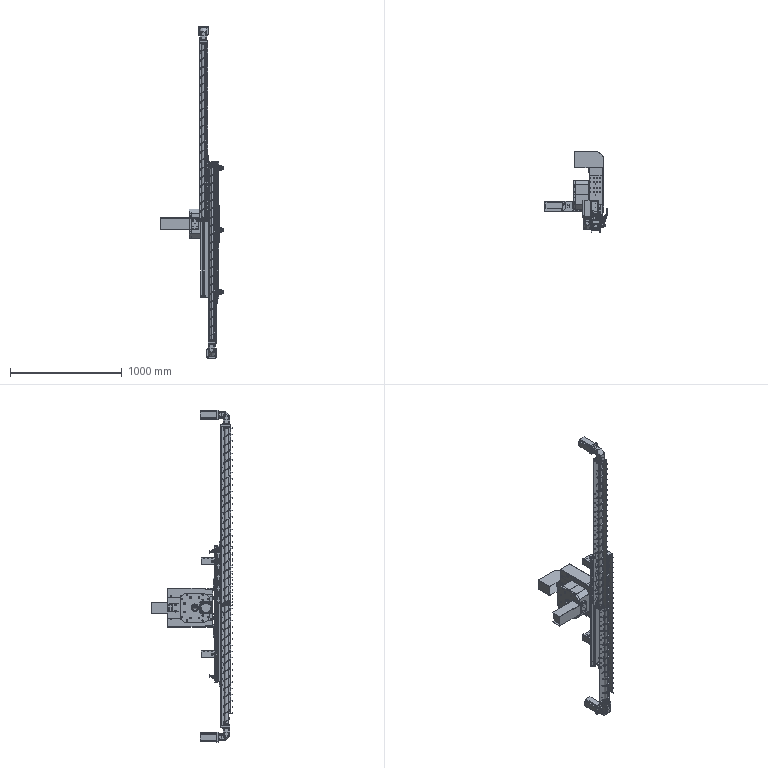Part | SolidWorks | features InContextFeatHolder 30, CenterOfMass 1 | 308 solids | 23655 faces | volume 27603448 mm3 | plane 12302 | cylinder 8570 | cone 1647 | spline 734 | torus 288 | sphere 114 | commonest cylinder face diameters 1 x1364 0.2 x612 2 x530 4.2 x396 4.06 x384 6 x378